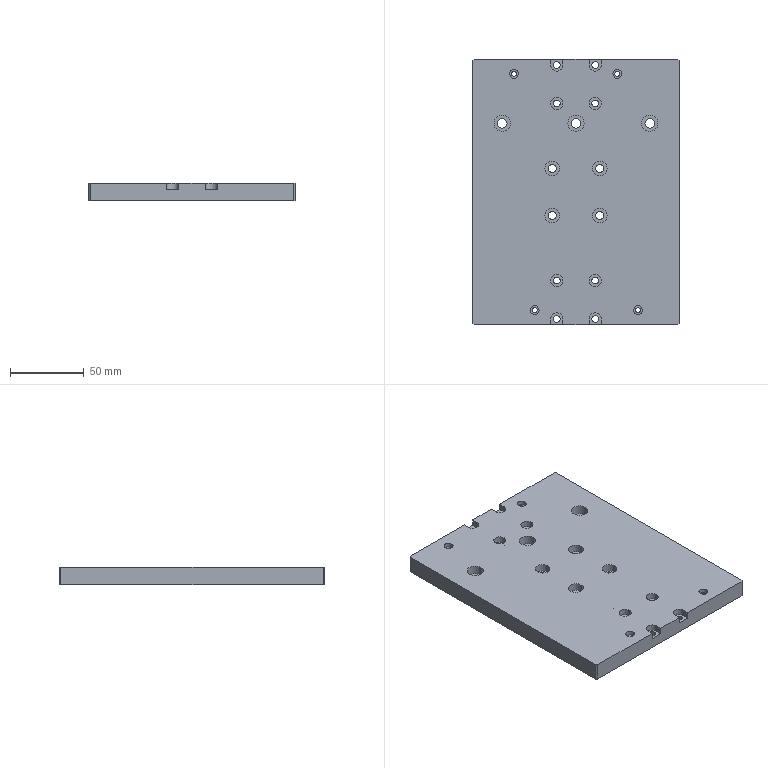Part | SolidWorks | features HoleWzd 7, Chamfer 1, Extrusion 1, ICE 1 | 1 solid | 145 faces | box 140 x 180 x 12 mm | volume 292625 mm3 | cylinder 92 | plane 41 | cone 12 | commonest cylinder face diameters 4.5 x16 8.2 x12 3.4 x8 5 x8 5.5 x8 6 x8